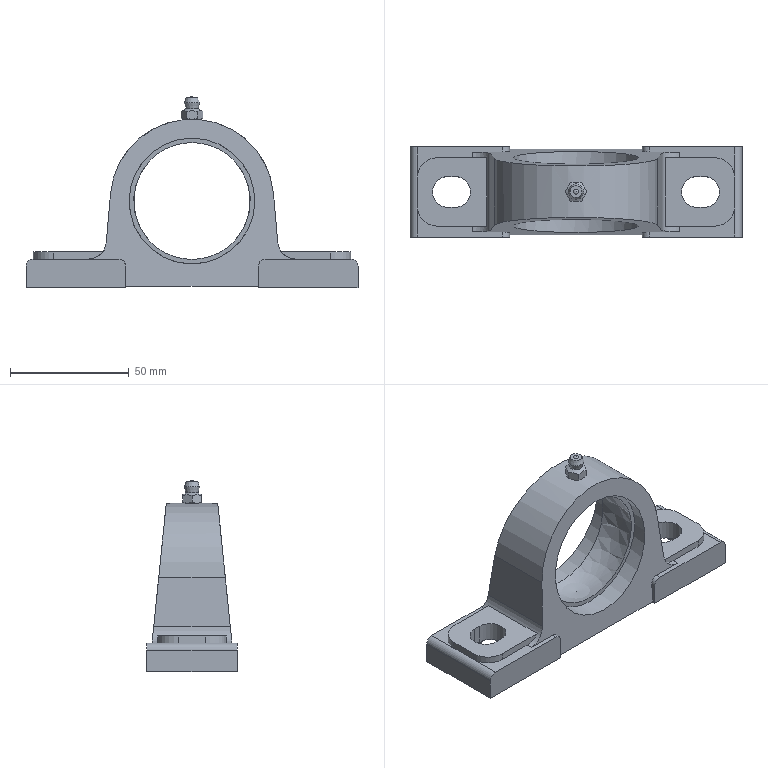Part | STEP file | 02288023_02 | 1 solid | 82 faces | box 140 x 38 x 80.599 mm | volume 93957 mm3 | plane 51 | cylinder 20 | cone 9 | sphere 2 | commonest cylinder face diameters 6 x6 13 x4 17.346 x4 15 x2 53.06 x2 6.37 x1